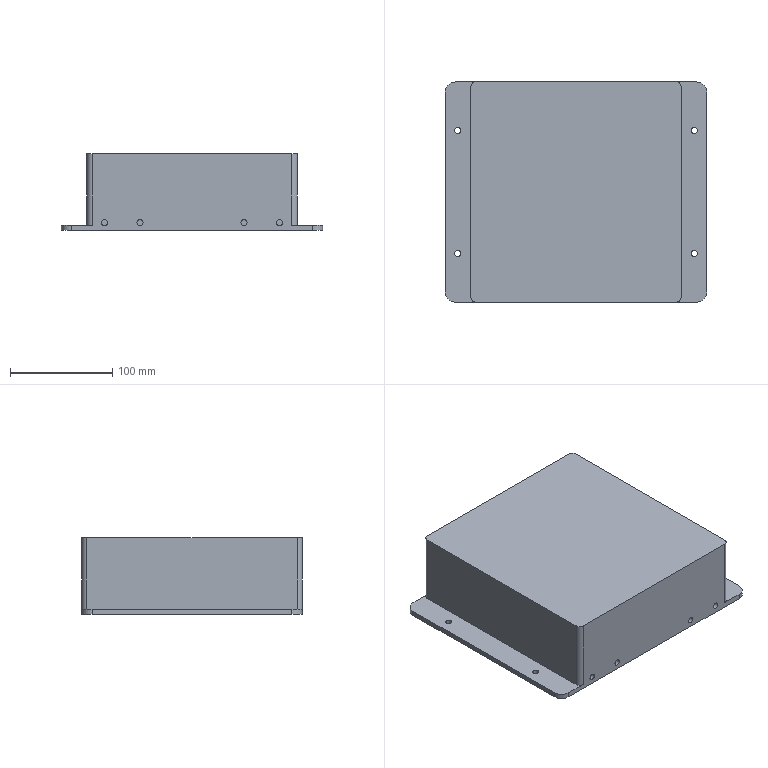Part | 1 solid | 46 faces | box 255 x 215 x 75 mm | volume 559118 mm3 | cylinder 29 | plane 17 | commonest cylinder face diameters 6 x16 10 x9 20 x4
STEP:
#1=CARTESIAN_POINT('',(102.5,102.5,0.));
#2=VERTEX_POINT('',#1);
#3=CARTESIAN_POINT('',(102.5,-102.5,0.));
#4=VERTEX_POINT('',#3);
#5=CARTESIAN_POINT('',(102.5,102.5,0.));
#6=DIRECTION('',(0.,-1.,0.));
#7=VECTOR('',#6,1000.);
#8=LINE('',#5,#7);
#9=EDGE_CURVE('',#2,#4,#8,.T.);
#10=ORIENTED_EDGE('',*,*,#9,.F.);
#11=CARTESIAN_POINT('',(97.5,107.5,0.));
#12=VERTEX_POINT('',#11);
#13=CARTESIAN_POINT('',(97.5,102.5,0.));
#14=DIRECTION('',(0.,0.,1.));
#15=DIRECTION('',(1.,0.,0.));
#16=AXIS2_PLACEMENT_3D('',#13,#14,#15);
#17=CIRCLE('',#16,5.);
#18=EDGE_CURVE('',#2,#12,#17,.T.);
#19=ORIENTED_EDGE('',*,*,#18,.T.);
#20=CARTESIAN_POINT('',(-97.5,107.5,0.));
#21=VERTEX_POINT('',#20);
#22=CARTESIAN_POINT('',(-97.5,107.5,0.));
#23=DIRECTION('',(1.,0.,0.));
#24=VECTOR('',#23,1000.);
#25=LINE('',#22,#24);
#26=EDGE_CURVE('',#21,#12,#25,.T.);
#27=ORIENTED_EDGE('',*,*,#26,.F.);
#28=CARTESIAN_POINT('',(-102.5,102.5,0.));
#29=VERTEX_POINT('',#28);
#30=CARTESIAN_POINT('',(-97.5,102.5,0.));
#31=DIRECTION('',(0.,0.,1.));
#32=DIRECTION('',(0.,1.,0.));
#33=AXIS2_PLACEMENT_3D('',#30,#31,#32);
#34=CIRCLE('',#33,5.);
#35=EDGE_CURVE('',#21,#29,#34,.T.);
#36=ORIENTED_EDGE('',*,*,#35,.T.);
#37=CARTESIAN_POINT('',(-102.5,-102.5,0.));
#38=VERTEX_POINT('',#37);
#39=CARTESIAN_POINT('',(-102.5,-102.5,0.));
#40=DIRECTION('',(0.,1.,0.));
#41=VECTOR('',#40,1000.);
#42=LINE('',#39,#41);
#43=EDGE_CURVE('',#38,#29,#42,.T.);
#44=ORIENTED_EDGE('',*,*,#43,.F.);
#45=CARTESIAN_POINT('',(-97.5,-107.5,0.));
#46=VERTEX_POINT('',#45);
#47=CARTESIAN_POINT('',(-97.5,-102.5,0.));
#48=DIRECTION('',(0.,0.,1.));
#49=DIRECTION('',(-1.,0.,0.));
#50=AXIS2_PLACEMENT_3D('',#47,#48,#49);
#51=CIRCLE('',#50,5.);
#52=EDGE_CURVE('',#38,#46,#51,.T.);
#53=ORIENTED_EDGE('',*,*,#52,.T.);
#54=CARTESIAN_POINT('',(97.5,-107.5,0.));
#55=VERTEX_POINT('',#54);
#56=CARTESIAN_POINT('',(97.5,-107.5,0.));
#57=DIRECTION('',(-1.,0.,0.));
#58=VECTOR('',#57,1000.);
#59=LINE('',#56,#58);
#60=EDGE_CURVE('',#55,#46,#59,.T.);
#61=ORIENTED_EDGE('',*,*,#60,.F.);
#62=CARTESIAN_POINT('',(97.5,-102.5,0.));
#63=DIRECTION('',(0.,0.,1.));
#64=DIRECTION('',(0.,-1.,0.));
#65=AXIS2_PLACEMENT_3D('',#62,#63,#64);
#66=CIRCLE('',#65,5.);
#67=EDGE_CURVE('',#55,#4,#66,.T.);
#68=ORIENTED_EDGE('',*,*,#67,.T.);
#69=EDGE_LOOP('',(#10,#19,#27,#36,#44,#53,#61,#68));
#70=FACE_BOUND('',#69,.T.);
#71=CARTESIAN_POINT('',(0.,5.,0.));
#72=DIRECTION('',(0.,0.,-1.));
#73=DIRECTION('',(1.,0.,0.));
#74=AXIS2_PLACEMENT_3D('',#71,#72,#73);
#75=PLANE('',#74);
#76=ADVANCED_FACE('',(#70),#75,.F.);
#77=CARTESIAN_POINT('',(97.5,-107.5,-70.));
#78=VERTEX_POINT('',#77);
#79=CARTESIAN_POINT('',(97.5,-107.5,-70.));
#80=DIRECTION('',(0.,0.,1.));
#81=VECTOR('',#80,1000.);
#82=LINE('',#79,#81);
#83=EDGE_CURVE('',#78,#55,#82,.T.);
#84=ORIENTED_EDGE('',*,*,#83,.F.);
#85=CARTESIAN_POINT('',(102.5,-102.5,-70.));
#86=VERTEX_POINT('',#85);
#87=CARTESIAN_POINT('',(97.5,-102.5,-70.));
#88=DIRECTION('',(0.,0.,-1.));
#89=DIRECTION('',(1.,0.,0.));
#90=AXIS2_PLACEMENT_3D('',#87,#88,#89);
#91=CIRCLE('',#90,5.);
#92=EDGE_CURVE('',#86,#78,#91,.T.);
#93=ORIENTED_EDGE('',*,*,#92,.F.);
#94=CARTESIAN_POINT('',(102.5,-102.5,-70.));
#95=DIRECTION('',(0.,0.,1.));
#96=VECTOR('',#95,1000.);
#97=LINE('',#94,#96);
#98=EDGE_CURVE('',#86,#4,#97,.T.);
#99=ORIENTED_EDGE('',*,*,#98,.T.);
#100=ORIENTED_EDGE('',*,*,#67,.F.);
#101=EDGE_LOOP('',(#84,#93,#99,#100));
#102=FACE_BOUND('',#101,.T.);
#103=CARTESIAN_POINT('',(97.5,-102.5,-172.77));
#104=DIRECTION('',(0.,0.,1.));
#105=DIRECTION('',(0.,1.,0.));
#106=AXIS2_PLACEMENT_3D('',#103,#104,#105);
#107=CYLINDRICAL_SURFACE('',#106,5.);
#108=ADVANCED_FACE('',(#102),#107,.T.);
#109=CARTESIAN_POINT('',(102.5,102.5,-70.));
#110=VERTEX_POINT('',#109);
#111=CARTESIAN_POINT('',(102.5,102.5,-70.));
#112=DIRECTION('',(0.,-1.,0.));
#113=VECTOR('',#112,1000.);
#114=LINE('',#111,#113);
#115=EDGE_CURVE('',#110,#86,#114,.T.);
#116=ORIENTED_EDGE('',*,*,#115,.F.);
#117=CARTESIAN_POINT('',(102.5,102.5,-70.));
#118=DIRECTION('',(0.,0.,1.));
#119=VECTOR('',#118,1000.);
#120=LINE('',#117,#119);
#121=EDGE_CURVE('',#110,#2,#120,.T.);
#122=ORIENTED_EDGE('',*,*,#121,.T.);
#123=ORIENTED_EDGE('',*,*,#9,.T.);
#124=ORIENTED_EDGE('',*,*,#98,.F.);
#125=EDGE_LOOP('',(#116,#122,#123,#124));
#126=FACE_BOUND('',#125,.T.);
#127=CARTESIAN_POINT('',(102.5,107.5,0.));
#128=DIRECTION('',(1.,0.,0.));
#129=DIRECTION('',(0.,1.,0.));
#130=AXIS2_PLACEMENT_3D('',#127,#128,#129);
#131=PLANE('',#130);
#132=ADVANCED_FACE('',(#126),#131,.T.);
#133=ORIENTED_EDGE('',*,*,#121,.F.);
#134=CARTESIAN_POINT('',(97.5,107.5,-70.));
#135=VERTEX_POINT('',#134);
#136=CARTESIAN_POINT('',(97.5,102.5,-70.));
#137=DIRECTION('',(0.,0.,-1.));
#138=DIRECTION('',(0.,1.,0.));
#139=AXIS2_PLACEMENT_3D('',#136,#137,#138);
#140=CIRCLE('',#139,5.);
#141=EDGE_CURVE('',#135,#110,#140,.T.);
#142=ORIENTED_EDGE('',*,*,#141,.F.);
#143=CARTESIAN_POINT('',(97.5,107.5,-70.));
#144=DIRECTION('',(0.,0.,1.));
#145=VECTOR('',#144,1000.);
#146=LINE('',#143,#145);
#147=EDGE_CURVE('',#135,#12,#146,.T.);
#148=ORIENTED_EDGE('',*,*,#147,.T.);
#149=ORIENTED_EDGE('',*,*,#18,.F.);
#150=EDGE_LOOP('',(#133,#142,#148,#149));
#151=FACE_BOUND('',#150,.T.);
#152=CARTESIAN_POINT('',(97.5,102.5,-172.77));
#153=DIRECTION('',(0.,0.,1.));
#154=DIRECTION('',(-1.,0.,0.));
#155=AXIS2_PLACEMENT_3D('',#152,#153,#154);
#156=CYLINDRICAL_SURFACE('',#155,5.);
#157=ADVANCED_FACE('',(#151),#156,.T.);
#158=ORIENTED_EDGE('',*,*,#26,.T.);
#159=ORIENTED_EDGE('',*,*,#147,.F.);
#160=CARTESIAN_POINT('',(117.5,107.5,-70.));
#161=VERTEX_POINT('',#160);
#162=CARTESIAN_POINT('',(97.5,107.5,-70.));
#163=DIRECTION('',(1.,0.,0.));
#164=VECTOR('',#163,1000.);
#165=LINE('',#162,#164);
#166=EDGE_CURVE('',#135,#161,#165,.T.);
#167=ORIENTED_EDGE('',*,*,#166,.T.);
#168=CARTESIAN_POINT('',(117.5,107.5,-75.));
#169=VERTEX_POINT('',#168);
#170=CARTESIAN_POINT('',(117.5,107.5,-75.));
#171=DIRECTION('',(0.,0.,1.));
#172=VECTOR('',#171,1000.);
#173=LINE('',#170,#172);
#174=EDGE_CURVE('',#169,#161,#173,.T.);
#175=ORIENTED_EDGE('',*,*,#174,.F.);
#176=CARTESIAN_POINT('',(70.,107.5,-75.));
#177=VERTEX_POINT('',#176);
#178=CARTESIAN_POINT('',(70.,107.5,-75.));
#179=DIRECTION('',(1.,0.,0.));
#180=VECTOR('',#179,1000.);
#181=LINE('',#178,#180);
#182=EDGE_CURVE('',#177,#169,#181,.T.);
#183=ORIENTED_EDGE('',*,*,#182,.F.);
#184=CARTESIAN_POINT('',(70.,107.5,-70.));
#185=VERTEX_POINT('',#184);
#186=CARTESIAN_POINT('',(70.,107.5,-75.));
#187=DIRECTION('',(0.,0.,1.));
#188=VECTOR('',#187,1000.);
#189=LINE('',#186,#188);
#190=EDGE_CURVE('',#177,#185,#189,.T.);
#191=ORIENTED_EDGE('',*,*,#190,.T.);
#192=CARTESIAN_POINT('',(60.,107.5,-70.));
#193=VERTEX_POINT('',#192);
#194=CARTESIAN_POINT('',(65.,107.5,-70.));
#195=DIRECTION('',(0.,1.,0.));
#196=DIRECTION('',(-1.,0.,0.));
#197=AXIS2_PLACEMENT_3D('',#194,#195,#196);
#198=CIRCLE('',#197,5.);
#199=EDGE_CURVE('',#193,#185,#198,.T.);
#200=ORIENTED_EDGE('',*,*,#199,.F.);
#201=CARTESIAN_POINT('',(60.,107.5,-75.));
#202=VERTEX_POINT('',#201);
#203=CARTESIAN_POINT('',(60.,107.5,-75.));
#204=DIRECTION('',(0.,0.,1.));
#205=VECTOR('',#204,1000.);
#206=LINE('',#203,#205);
#207=EDGE_CURVE('',#202,#193,#206,.T.);
#208=ORIENTED_EDGE('',*,*,#207,.F.);
#209=CARTESIAN_POINT('',(-117.5,107.5,-75.));
#210=VERTEX_POINT('',#209);
#211=CARTESIAN_POINT('',(-117.5,107.5,-75.));
#212=DIRECTION('',(1.,0.,0.));
#213=VECTOR('',#212,1000.);
#214=LINE('',#211,#213);
#215=EDGE_CURVE('',#210,#202,#214,.T.);
#216=ORIENTED_EDGE('',*,*,#215,.F.);
#217=CARTESIAN_POINT('',(-117.5,107.5,-70.));
#218=VERTEX_POINT('',#217);
#219=CARTESIAN_POINT('',(-117.5,107.5,-75.));
#220=DIRECTION('',(0.,0.,1.));
#221=VECTOR('',#220,1000.);
#222=LINE('',#219,#221);
#223=EDGE_CURVE('',#210,#218,#222,.T.);
#224=ORIENTED_EDGE('',*,*,#223,.T.);
#225=CARTESIAN_POINT('',(-97.5,107.5,-70.));
#226=VERTEX_POINT('',#225);
#227=CARTESIAN_POINT('',(-117.5,107.5,-70.));
#228=DIRECTION('',(1.,0.,0.));
#229=VECTOR('',#228,1000.);
#230=LINE('',#227,#229);
#231=EDGE_CURVE('',#218,#226,#230,.T.);
#232=ORIENTED_EDGE('',*,*,#231,.T.);
#233=CARTESIAN_POINT('',(-97.5,107.5,-70.));
#234=DIRECTION('',(0.,0.,1.));
#235=VECTOR('',#234,1000.);
#236=LINE('',#233,#235);
#237=EDGE_CURVE('',#226,#21,#236,.T.);
#238=ORIENTED_EDGE('',*,*,#237,.T.);
#239=EDGE_LOOP('',(#158,#159,#167,#175,#183,#191,#200,#208,#216,#224,#232,#238));
#240=FACE_BOUND('',#239,.T.);
#241=CARTESIAN_POINT('',(-102.5,107.5,0.));
#242=DIRECTION('',(0.,1.,0.));
#243=DIRECTION('',(-1.,0.,0.));
#244=AXIS2_PLACEMENT_3D('',#241,#242,#243);
#245=PLANE('',#244);
#246=ADVANCED_FACE('',(#240),#245,.T.);
#247=ORIENTED_EDGE('',*,*,#237,.F.);
#248=CARTESIAN_POINT('',(-102.5,102.5,-70.));
#249=VERTEX_POINT('',#248);
#250=CARTESIAN_POINT('',(-97.5,102.5,-70.));
#251=DIRECTION('',(0.,0.,-1.));
#252=DIRECTION('',(-1.,0.,0.));
#253=AXIS2_PLACEMENT_3D('',#250,#251,#252);
#254=CIRCLE('',#253,5.);
#255=EDGE_CURVE('',#249,#226,#254,.T.);
#256=ORIENTED_EDGE('',*,*,#255,.F.);
#257=CARTESIAN_POINT('',(-102.5,102.5,-70.));
#258=DIRECTION('',(0.,0.,1.));
#259=VECTOR('',#258,1000.);
#260=LINE('',#257,#259);
#261=EDGE_CURVE('',#249,#29,#260,.T.);
#262=ORIENTED_EDGE('',*,*,#261,.T.);
#263=ORIENTED_EDGE('',*,*,#35,.F.);
#264=EDGE_LOOP('',(#247,#256,#262,#263));
#265=FACE_BOUND('',#264,.T.);
#266=CARTESIAN_POINT('',(-97.5,102.5,-172.77));
#267=DIRECTION('',(0.,0.,1.));
#268=DIRECTION('',(0.,-1.,0.));
#269=AXIS2_PLACEMENT_3D('',#266,#267,#268);
#270=CYLINDRICAL_SURFACE('',#269,5.);
#271=ADVANCED_FACE('',(#265),#270,.T.);
#272=ORIENTED_EDGE('',*,*,#43,.T.);
#273=ORIENTED_EDGE('',*,*,#261,.F.);
#274=CARTESIAN_POINT('',(-102.5,-102.5,-70.));
#275=VERTEX_POINT('',#274);
#276=CARTESIAN_POINT('',(-102.5,-102.5,-70.));
#277=DIRECTION('',(0.,1.,0.));
#278=VECTOR('',#277,1000.);
#279=LINE('',#276,#278);
#280=EDGE_CURVE('',#275,#249,#279,.T.);
#281=ORIENTED_EDGE('',*,*,#280,.F.);
#282=CARTESIAN_POINT('',(-102.5,-102.5,-70.));
#283=DIRECTION('',(0.,0.,1.));
#284=VECTOR('',#283,1000.);
#285=LINE('',#282,#284);
#286=EDGE_CURVE('',#275,#38,#285,.T.);
#287=ORIENTED_EDGE('',*,*,#286,.T.);
#288=EDGE_LOOP('',(#272,#273,#281,#287));
#289=FACE_BOUND('',#288,.T.);
#290=CARTESIAN_POINT('',(-102.5,-97.5,0.));
#291=DIRECTION('',(-1.,0.,0.));
#292=DIRECTION('',(0.,-1.,0.));
#293=AXIS2_PLACEMENT_3D('',#290,#291,#292);
#294=PLANE('',#293);
#295=ADVANCED_FACE('',(#289),#294,.T.);
#296=ORIENTED_EDGE('',*,*,#286,.F.);
#297=CARTESIAN_POINT('',(-97.5,-107.5,-70.));
#298=VERTEX_POINT('',#297);
#299=CARTESIAN_POINT('',(-97.5,-102.5,-70.));
#300=DIRECTION('',(0.,0.,-1.));
#301=DIRECTION('',(0.,-1.,0.));
#302=AXIS2_PLACEMENT_3D('',#299,#300,#301);
#303=CIRCLE('',#302,5.);
#304=EDGE_CURVE('',#298,#275,#303,.T.);
#305=ORIENTED_EDGE('',*,*,#304,.F.);
#306=CARTESIAN_POINT('',(-97.5,-107.5,-70.));
#307=DIRECTION('',(0.,0.,1.));
#308=VECTOR('',#307,1000.);
#309=LINE('',#306,#308);
#310=EDGE_CURVE('',#298,#46,#309,.T.);
#311=ORIENTED_EDGE('',*,*,#310,.T.);
#312=ORIENTED_EDGE('',*,*,#52,.F.);
#313=EDGE_LOOP('',(#296,#305,#311,#312));
#314=FACE_BOUND('',#313,.T.);
#315=CARTESIAN_POINT('',(-97.5,-102.5,-172.77));
#316=DIRECTION('',(0.,0.,1.));
#317=DIRECTION('',(1.,0.,0.));
#318=AXIS2_PLACEMENT_3D('',#315,#316,#317);
#319=CYLINDRICAL_SURFACE('',#318,5.);
#320=ADVANCED_FACE('',(#314),#319,.T.);
#321=ORIENTED_EDGE('',*,*,#60,.T.);
#322=ORIENTED_EDGE('',*,*,#310,.F.);
#323=CARTESIAN_POINT('',(-117.5,-107.5,-70.));
#324=VERTEX_POINT('',#323);
#325=CARTESIAN_POINT('',(-97.5,-107.5,-70.));
#326=DIRECTION('',(-1.,0.,0.));
#327=VECTOR('',#326,1000.);
#328=LINE('',#325,#327);
#329=EDGE_CURVE('',#298,#324,#328,.T.);
#330=ORIENTED_EDGE('',*,*,#329,.T.);
#331=CARTESIAN_POINT('',(-117.5,-107.5,-75.));
#332=VERTEX_POINT('',#331);
#333=CARTESIAN_POINT('',(-117.5,-107.5,-75.));
#334=DIRECTION('',(0.,0.,1.));
#335=VECTOR('',#334,1000.);
#336=LINE('',#333,#335);
#337=EDGE_CURVE('',#332,#324,#336,.T.);
#338=ORIENTED_EDGE('',*,*,#337,.F.);
#339=CARTESIAN_POINT('',(117.5,-107.5,-75.));
#340=VERTEX_POINT('',#339);
#341=CARTESIAN_POINT('',(117.5,-107.5,-75.));
#342=DIRECTION('',(-1.,0.,0.));
#343=VECTOR('',#342,1000.);
#344=LINE('',#341,#343);
#345=EDGE_CURVE('',#340,#332,#344,.T.);
#346=ORIENTED_EDGE('',*,*,#345,.F.);
#347=CARTESIAN_POINT('',(117.5,-107.5,-70.));
#348=VERTEX_POINT('',#347);
#349=CARTESIAN_POINT('',(117.5,-107.5,-75.));
#350=DIRECTION('',(0.,0.,1.));
#351=VECTOR('',#350,1000.);
#352=LINE('',#349,#351);
#353=EDGE_CURVE('',#340,#348,#352,.T.);
#354=ORIENTED_EDGE('',*,*,#353,.T.);
#355=CARTESIAN_POINT('',(117.5,-107.5,-70.));
#356=DIRECTION('',(-1.,0.,0.));
#357=VECTOR('',#356,1000.);
#358=LINE('',#355,#357);
#359=EDGE_CURVE('',#348,#78,#358,.T.);
#360=ORIENTED_EDGE('',*,*,#359,.T.);
#361=ORIENTED_EDGE('',*,*,#83,.T.);
#362=EDGE_LOOP('',(#321,#322,#330,#338,#346,#354,#360,#361));
#363=FACE_BOUND('',#362,.T.);
#364=CARTESIAN_POINT('',(-82.25,-107.5,-67.35));
#365=VERTEX_POINT('',#364);
#366=CARTESIAN_POINT('',(-88.25,-107.5,-67.35));
#367=VERTEX_POINT('',#366);
#368=CARTESIAN_POINT('',(-85.25,-107.5,-67.35));
#369=DIRECTION('',(0.,-1.,0.));
#370=DIRECTION('',(1.,0.,0.));
#371=AXIS2_PLACEMENT_3D('',#368,#369,#370);
#372=CIRCLE('',#371,3.);
#373=EDGE_CURVE('',#365,#367,#372,.T.);
#374=ORIENTED_EDGE('',*,*,#373,.F.);
#375=CARTESIAN_POINT('',(-85.25,-107.5,-67.35));
#376=DIRECTION('',(0.,-1.,0.));
#377=DIRECTION('',(-1.,0.,0.));
#378=AXIS2_PLACEMENT_3D('',#375,#376,#377);
#379=CIRCLE('',#378,3.);
#380=EDGE_CURVE('',#367,#365,#379,.T.);
#381=ORIENTED_EDGE('',*,*,#380,.F.);
#382=EDGE_LOOP('',(#374,#381));
#383=FACE_BOUND('',#382,.T.);
#384=CARTESIAN_POINT('',(53.75,-107.5,-67.35));
#385=VERTEX_POINT('',#384);
#386=CARTESIAN_POINT('',(47.75,-107.5,-67.35));
#387=VERTEX_POINT('',#386);
#388=CARTESIAN_POINT('',(50.75,-107.5,-67.35));
#389=DIRECTION('',(0.,-1.,0.));
#390=DIRECTION('',(1.,0.,0.));
#391=AXIS2_PLACEMENT_3D('',#388,#389,#390);
#392=CIRCLE('',#391,3.);
#393=EDGE_CURVE('',#385,#387,#392,.T.);
#394=ORIENTED_EDGE('',*,*,#393,.F.);
#395=CARTESIAN_POINT('',(50.75,-107.5,-67.35));
#396=DIRECTION('',(0.,-1.,0.));
#397=DIRECTION('',(-1.,0.,0.));
#398=AXIS2_PLACEMENT_3D('',#395,#396,#397);
#399=CIRCLE('',#398,3.);
#400=EDGE_CURVE('',#387,#385,#399,.T.);
#401=ORIENTED_EDGE('',*,*,#400,.F.);
#402=EDGE_LOOP('',(#394,#401));
#403=FACE_BOUND('',#402,.T.);
#404=CARTESIAN_POINT('',(88.25,-107.5,-67.35));
#405=VERTEX_POINT('',#404);
#406=CARTESIAN_POINT('',(82.25,-107.5,-67.35));
#407=VERTEX_POINT('',#406);
#408=CARTESIAN_POINT('',(85.25,-107.5,-67.35));
#409=DIRECTION('',(0.,-1.,0.));
#410=DIRECTION('',(1.,0.,0.));
#411=AXIS2_PLACEMENT_3D('',#408,#409,#410);
#412=CIRCLE('',#411,3.);
#413=EDGE_CURVE('',#405,#407,#412,.T.);
#414=ORIENTED_EDGE('',*,*,#413,.F.);
#415=CARTESIAN_POINT('',(85.25,-107.5,-67.35));
#416=DIRECTION('',(0.,-1.,0.));
#417=DIRECTION('',(-1.,0.,0.));
#418=AXIS2_PLACEMENT_3D('',#415,#416,#417);
#419=CIRCLE('',#418,3.);
#420=EDGE_CURVE('',#407,#405,#419,.T.);
#421=ORIENTED_EDGE('',*,*,#420,.F.);
#422=EDGE_LOOP('',(#414,#421));
#423=FACE_BOUND('',#422,.T.);
#424=CARTESIAN_POINT('',(-47.75,-107.5,-67.35));
#425=VERTEX_POINT('',#424);
#426=CARTESIAN_POINT('',(-53.75,-107.5,-67.35));
#427=VERTEX_POINT('',#426);
#428=CARTESIAN_POINT('',(-50.75,-107.5,-67.35));
#429=DIRECTION('',(0.,-1.,0.));
#430=DIRECTION('',(1.,0.,0.));
#431=AXIS2_PLACEMENT_3D('',#428,#429,#430);
#432=CIRCLE('',#431,3.);
#433=EDGE_CURVE('',#425,#427,#432,.T.);
#434=ORIENTED_EDGE('',*,*,#433,.F.);
#435=CARTESIAN_POINT('',(-50.75,-107.5,-67.35));
#436=DIRECTION('',(0.,-1.,0.));
#437=DIRECTION('',(-1.,0.,0.));
#438=AXIS2_PLACEMENT_3D('',#435,#436,#437);
#439=CIRCLE('',#438,3.);
#440=EDGE_CURVE('',#427,#425,#439,.T.);
#441=ORIENTED_EDGE('',*,*,#440,.F.);
#442=EDGE_LOOP('',(#434,#441));
#443=FACE_BOUND('',#442,.T.);
#444=CARTESIAN_POINT('',(102.5,-107.5,0.));
#445=DIRECTION('',(0.,-1.,0.));
#446=DIRECTION('',(1.,0.,0.));
#447=AXIS2_PLACEMENT_3D('',#444,#445,#446);
#448=PLANE('',#447);
#449=ADVANCED_FACE('',(#363,#383,#403,#423,#443),#448,.T.);
#450=CARTESIAN_POINT('',(-47.75,-102.5,-67.35));
#451=VERTEX_POINT('',#450);
#452=CARTESIAN_POINT('',(-47.75,-107.5,-67.35));
#453=DIRECTION('',(0.,1.,0.));
#454=VECTOR('',#453,1000.);
#455=LINE('',#452,#454);
#456=EDGE_CURVE('',#451,#425,#455,.F.);
#457=ORIENTED_EDGE('',*,*,#456,.F.);
#458=CARTESIAN_POINT('',(-53.75,-102.5,-67.35));
#459=VERTEX_POINT('',#458);
#460=CARTESIAN_POINT('',(-50.75,-102.5,-67.35));
#461=DIRECTION('',(0.,-1.,0.));
#462=DIRECTION('',(-1.,0.,0.));
#463=AXIS2_PLACEMENT_3D('',#460,#461,#462);
#464=CIRCLE('',#463,3.);
#465=EDGE_CURVE('',#459,#451,#464,.T.);
#466=ORIENTED_EDGE('',*,*,#465,.F.);
#467=CARTESIAN_POINT('',(-53.75,-107.5,-67.35));
#468=DIRECTION('',(0.,1.,0.));
#469=VECTOR('',#468,1000.);
#470=LINE('',#467,#469);
#471=EDGE_CURVE('',#459,#427,#470,.F.);
#472=ORIENTED_EDGE('',*,*,#471,.T.);
#473=ORIENTED_EDGE('',*,*,#440,.T.);
#474=EDGE_LOOP('',(#457,#466,#472,#473));
#475=FACE_BOUND('',#474,.T.);
#476=CARTESIAN_POINT('',(-50.75,-107.5,-67.35));
#477=DIRECTION('',(0.,-1.,0.));
#478=DIRECTION('',(1.,0.,0.));
#479=AXIS2_PLACEMENT_3D('',#476,#477,#478);
#480=CYLINDRICAL_SURFACE('',#479,3.);
#481=ADVANCED_FACE('',(#475),#480,.F.);
#482=ORIENTED_EDGE('',*,*,#471,.F.);
#483=CARTESIAN_POINT('',(-50.75,-102.5,-67.35));
#484=DIRECTION('',(0.,-1.,0.));
#485=DIRECTION('',(1.,0.,0.));
#486=AXIS2_PLACEMENT_3D('',#483,#484,#485);
#487=CIRCLE('',#486,3.);
#488=EDGE_CURVE('',#451,#459,#487,.T.);
#489=ORIENTED_EDGE('',*,*,#488,.F.);
#490=ORIENTED_EDGE('',*,*,#456,.T.);
#491=ORIENTED_EDGE('',*,*,#433,.T.);
#492=EDGE_LOOP('',(#482,#489,#490,#491));
#493=FACE_BOUND('',#492,.T.);
#494=CARTESIAN_POINT('',(-50.75,-107.5,-67.35));
#495=DIRECTION('',(0.,-1.,0.));
#496=DIRECTION('',(1.,0.,0.));
#497=AXIS2_PLACEMENT_3D('',#494,#495,#496);
#498=CYLINDRICAL_SURFACE('',#497,3.);
#499=ADVANCED_FACE('',(#493),#498,.F.);
#500=CARTESIAN_POINT('',(92.5,-102.5,-5.));
#501=VERTEX_POINT('',#500);
#502=CARTESIAN_POINT('',(-92.5,-102.5,-5.));
#503=VERTEX_POINT('',#502);
#504=CARTESIAN_POINT('',(92.5,-102.5,-5.));
#505=DIRECTION('',(-1.,0.,0.));
#506=VECTOR('',#505,1000.);
#507=LINE('',#504,#506);
#508=EDGE_CURVE('',#501,#503,#507,.T.);
#509=ORIENTED_EDGE('',*,*,#508,.F.);
#510=CARTESIAN_POINT('',(92.5,-102.5,-75.));
#511=VERTEX_POINT('',#510);
#512=CARTESIAN_POINT('',(92.5,-102.5,-75.));
#513=DIRECTION('',(0.,0.,1.));
#514=VECTOR('',#513,1000.);
#515=LINE('',#512,#514);
#516=EDGE_CURVE('',#511,#501,#515,.T.);
#517=ORIENTED_EDGE('',*,*,#516,.F.);
#518=CARTESIAN_POINT('',(-92.5,-102.5,-75.));
#519=VERTEX_POINT('',#518);
#520=CARTESIAN_POINT('',(92.5,-102.5,-75.));
#521=DIRECTION('',(-1.,0.,0.));
#522=VECTOR('',#521,1000.);
#523=LINE('',#520,#522);
#524=EDGE_CURVE('',#511,#519,#523,.T.);
#525=ORIENTED_EDGE('',*,*,#524,.T.);
#526=CARTESIAN_POINT('',(-92.5,-102.5,-75.));
#527=DIRECTION('',(0.,0.,1.));
#528=VECTOR('',#527,1000.);
#529=LINE('',#526,#528);
#530=EDGE_CURVE('',#519,#503,#529,.T.);
#531=ORIENTED_EDGE('',*,*,#530,.T.);
#532=EDGE_LOOP('',(#509,#517,#525,#531));
#533=FACE_BOUND('',#532,.T.);
#534=CARTESIAN_POINT('',(-82.25,-102.5,-67.35));
#535=VERTEX_POINT('',#534);
#536=CARTESIAN_POINT('',(-88.25,-102.5,-67.35));
#537=VERTEX_POINT('',#536);
#538=CARTESIAN_POINT('',(-85.25,-102.5,-67.35));
#539=DIRECTION('',(0.,-1.,0.));
#540=DIRECTION('',(1.,0.,0.));
#541=AXIS2_PLACEMENT_3D('',#538,#539,#540);
#542=CIRCLE('',#541,3.);
#543=EDGE_CURVE('',#535,#537,#542,.T.);
#544=ORIENTED_EDGE('',*,*,#543,.T.);
#545=CARTESIAN_POINT('',(-85.25,-102.5,-67.35));
#546=DIRECTION('',(0.,-1.,0.));
#547=DIRECTION('',(-1.,0.,0.));
#548=AXIS2_PLACEMENT_3D('',#545,#546,#547);
#549=CIRCLE('',#548,3.);
#550=EDGE_CURVE('',#537,#535,#549,.T.);
#551=ORIENTED_EDGE('',*,*,#550,.T.);
#552=EDGE_LOOP('',(#544,#551));
#553=FACE_BOUND('',#552,.T.);
#554=CARTESIAN_POINT('',(53.75,-102.5,-67.35));
#555=VERTEX_POINT('',#554);
#556=CARTESIAN_POINT('',(47.75,-102.5,-67.35));
#557=VERTEX_POINT('',#556);
#558=CARTESIAN_POINT('',(50.75,-102.5,-67.35));
#559=DIRECTION('',(0.,-1.,0.));
#560=DIRECTION('',(1.,0.,0.));
#561=AXIS2_PLACEMENT_3D('',#558,#559,#560);
#562=CIRCLE('',#561,3.);
#563=EDGE_CURVE('',#555,#557,#562,.T.);
#564=ORIENTED_EDGE('',*,*,#563,.T.);
#565=CARTESIAN_POINT('',(50.75,-102.5,-67.35));
#566=DIRECTION('',(0.,-1.,0.));
#567=DIRECTION('',(-1.,0.,0.));
#568=AXIS2_PLACEMENT_3D('',#565,#566,#567);
#569=CIRCLE('',#568,3.);
#570=EDGE_CURVE('',#557,#555,#569,.T.);
#571=ORIENTED_EDGE('',*,*,#570,.T.);
#572=EDGE_LOOP('',(#564,#571));
#573=FACE_BOUND('',#572,.T.);
#574=CARTESIAN_POINT('',(88.25,-102.5,-67.35));
#575=VERTEX_POINT('',#574);
#576=CARTESIAN_POINT('',(82.25,-102.5,-67.35));
#577=VERTEX_POINT('',#576);
#578=CARTESIAN_POINT('',(85.25,-102.5,-67.35));
#579=DIRECTION('',(0.,-1.,0.));
#580=DIRECTION('',(1.,0.,0.));
#581=AXIS2_PLACEMENT_3D('',#578,#579,#580);
#582=CIRCLE('',#581,3.);
#583=EDGE_CURVE('',#575,#577,#582,.T.);
#584=ORIENTED_EDGE('',*,*,#583,.T.);
#585=CARTESIAN_POINT('',(85.25,-102.5,-67.35));
#586=DIRECTION('',(0.,-1.,0.));
#587=DIRECTION('',(-1.,0.,0.));
#588=AXIS2_PLACEMENT_3D('',#585,#586,#587);
#589=CIRCLE('',#588,3.);
#590=EDGE_CURVE('',#577,#575,#589,.T.);
#591=ORIENTED_EDGE('',*,*,#590,.T.);
#592=EDGE_LOOP('',(#584,#591));
#593=FACE_BOUND('',#592,.T.);
#594=ORIENTED_EDGE('',*,*,#488,.T.);
#595=ORIENTED_EDGE('',*,*,#465,.T.);
#596=EDGE_LOOP('',(#594,#595));
#597=FACE_BOUND('',#596,.T.);
#598=CARTESIAN_POINT('',(102.5,-102.5,0.));
#599=DIRECTION('',(0.,-1.,0.));
#600=DIRECTION('',(1.,0.,0.));
#601=AXIS2_PLACEMENT_3D('',#598,#599,#600);
#602=PLANE('',#601);
#603=ADVANCED_FACE('',(#533,#553,#573,#593,#597),#602,.F.);
#604=CARTESIAN_POINT('',(-82.25,-107.5,-67.35));
#605=DIRECTION('',(0.,1.,0.));
#606=VECTOR('',#605,1000.);
#607=LINE('',#604,#606);
#608=EDGE_CURVE('',#535,#365,#607,.F.);
#609=ORIENTED_EDGE('',*,*,#608,.F.);
#610=ORIENTED_EDGE('',*,*,#550,.F.);
#611=CARTESIAN_POINT('',(-88.25,-107.5,-67.35));
#612=DIRECTION('',(0.,1.,0.));
#613=VECTOR('',#612,1000.);
#614=LINE('',#611,#613);
#615=EDGE_CURVE('',#537,#367,#614,.F.);
#616=ORIENTED_EDGE('',*,*,#615,.T.);
#617=ORIENTED_EDGE('',*,*,#380,.T.);
#618=EDGE_LOOP('',(#609,#610,#616,#617));
#619=FACE_BOUND('',#618,.T.);
#620=CARTESIAN_POINT('',(-85.25,-107.5,-67.35));
#621=DIRECTION('',(0.,-1.,0.));
#622=DIRECTION('',(1.,0.,0.));
#623=AXIS2_PLACEMENT_3D('',#620,#621,#622);
#624=CYLINDRICAL_SURFACE('',#623,3.);
#625=ADVANCED_FACE('',(#619),#624,.F.);
#626=ORIENTED_EDGE('',*,*,#615,.F.);
#627=ORIENTED_EDGE('',*,*,#543,.F.);
#628=ORIENTED_EDGE('',*,*,#608,.T.);
#629=ORIENTED_EDGE('',*,*,#373,.T.);
#630=EDGE_LOOP('',(#626,#627,#628,#629));
#631=FACE_BOUND('',#630,.T.);
#632=CARTESIAN_POINT('',(-85.25,-107.5,-67.35));
#633=DIRECTION('',(0.,-1.,0.));
#634=DIRECTION('',(1.,0.,0.));
#635=AXIS2_PLACEMENT_3D('',#632,#633,#634);
#636=CYLINDRICAL_SURFACE('',#635,3.);
#637=ADVANCED_FACE('',(#631),#636,.F.);
#638=CARTESIAN_POINT('',(53.75,-107.5,-67.35));
#639=DIRECTION('',(0.,1.,0.));
#640=VECTOR('',#639,1000.);
#641=LINE('',#638,#640);
#642=EDGE_CURVE('',#555,#385,#641,.F.);
#643=ORIENTED_EDGE('',*,*,#642,.F.);
#644=ORIENTED_EDGE('',*,*,#570,.F.);
#645=CARTESIAN_POINT('',(47.75,-107.5,-67.35));
#646=DIRECTION('',(0.,1.,0.));
#647=VECTOR('',#646,1000.);
#648=LINE('',#645,#647);
#649=EDGE_CURVE('',#557,#387,#648,.F.);
#650=ORIENTED_EDGE('',*,*,#649,.T.);
#651=ORIENTED_EDGE('',*,*,#400,.T.);
#652=EDGE_LOOP('',(#643,#644,#650,#651));
#653=FACE_BOUND('',#652,.T.);
#654=CARTESIAN_POINT('',(50.75,-107.5,-67.35));
#655=DIRECTION('',(0.,-1.,0.));
#656=DIRECTION('',(1.,0.,0.));
#657=AXIS2_PLACEMENT_3D('',#654,#655,#656);
#658=CYLINDRICAL_SURFACE('',#657,3.);
#659=ADVANCED_FACE('',(#653),#658,.F.);
#660=ORIENTED_EDGE('',*,*,#649,.F.);
#661=ORIENTED_EDGE('',*,*,#563,.F.);
#662=ORIENTED_EDGE('',*,*,#642,.T.);
#663=ORIENTED_EDGE('',*,*,#393,.T.);
#664=EDGE_LOOP('',(#660,#661,#662,#663));
#665=FACE_BOUND('',#664,.T.);
#666=CARTESIAN_POINT('',(50.75,-107.5,-67.35));
#667=DIRECTION('',(0.,-1.,0.));
#668=DIRECTION('',(1.,0.,0.));
#669=AXIS2_PLACEMENT_3D('',#666,#667,#668);
#670=CYLINDRICAL_SURFACE('',#669,3.);
#671=ADVANCED_FACE('',(#665),#670,.F.);
#672=CARTESIAN_POINT('',(88.25,-107.5,-67.35));
#673=DIRECTION('',(0.,1.,0.));
#674=VECTOR('',#673,1000.);
#675=LINE('',#672,#674);
#676=EDGE_CURVE('',#575,#405,#675,.F.);
#677=ORIENTED_EDGE('',*,*,#676,.F.);
#678=ORIENTED_EDGE('',*,*,#590,.F.);
#679=CARTESIAN_POINT('',(82.25,-107.5,-67.35));
#680=DIRECTION('',(0.,1.,0.));
#681=VECTOR('',#680,1000.);
#682=LINE('',#679,#681);
#683=EDGE_CURVE('',#577,#407,#682,.F.);
#684=ORIENTED_EDGE('',*,*,#683,.T.);
#685=ORIENTED_EDGE('',*,*,#420,.T.);
#686=EDGE_LOOP('',(#677,#678,#684,#685));
#687=FACE_BOUND('',#686,.T.);
#688=CARTESIAN_POINT('',(85.25,-107.5,-67.35));
#689=DIRECTION('',(0.,-1.,0.));
#690=DIRECTION('',(1.,0.,0.));
#691=AXIS2_PLACEMENT_3D('',#688,#689,#690);
#692=CYLINDRICAL_SURFACE('',#691,3.);
#693=ADVANCED_FACE('',(#687),#692,.F.);
#694=ORIENTED_EDGE('',*,*,#683,.F.);
#695=ORIENTED_EDGE('',*,*,#583,.F.);
#696=ORIENTED_EDGE('',*,*,#676,.T.);
#697=ORIENTED_EDGE('',*,*,#413,.T.);
#698=EDGE_LOOP('',(#694,#695,#696,#697));
#699=FACE_BOUND('',#698,.T.);
#700=CARTESIAN_POINT('',(85.25,-107.5,-67.35));
#701=DIRECTION('',(0.,-1.,0.));
#702=DIRECTION('',(1.,0.,0.));
#703=AXIS2_PLACEMENT_3D('',#700,#701,#702);
#704=CYLINDRICAL_SURFACE('',#703,3.);
#705=ADVANCED_FACE('',(#699),#704,.F.);
#706=ORIENTED_EDGE('',*,*,#530,.F.);
#707=CARTESIAN_POINT('',(-97.5,-97.5,-75.));
#708=VERTEX_POINT('',#707);
#709=CARTESIAN_POINT('',(-92.5,-97.5,-75.));
#710=DIRECTION('',(0.,0.,1.));
#711=DIRECTION('',(-1.,0.,0.));
#712=AXIS2_PLACEMENT_3D('',#709,#710,#711);
#713=CIRCLE('',#712,5.);
#714=EDGE_CURVE('',#708,#519,#713,.T.);
#715=ORIENTED_EDGE('',*,*,#714,.F.);
#716=CARTESIAN_POINT('',(-97.5,-97.5,-5.));
#717=VERTEX_POINT('',#716);
#718=CARTESIAN_POINT('',(-97.5,-97.5,-75.));
#719=DIRECTION('',(0.,0.,1.));
#720=VECTOR('',#719,1000.);
#721=LINE('',#718,#720);
#722=EDGE_CURVE('',#708,#717,#721,.T.);
#723=ORIENTED_EDGE('',*,*,#722,.T.);
#724=CARTESIAN_POINT('',(-92.5,-97.5,-5.));
#725=DIRECTION('',(0.,0.,-1.));
#726=DIRECTION('',(0.,-1.,0.));
#727=AXIS2_PLACEMENT_3D('',#724,#725,#726);
#728=CIRCLE('',#727,5.);
#729=EDGE_CURVE('',#503,#717,#728,.T.);
#730=ORIENTED_EDGE('',*,*,#729,.F.);
#731=EDGE_LOOP('',(#706,#715,#723,#730));
#732=FACE_BOUND('',#731,.T.);
#733=CARTESIAN_POINT('',(-92.5,-97.5,-172.77));
#734=DIRECTION('',(0.,0.,1.));
#735=DIRECTION('',(1.,0.,0.));
#736=AXIS2_PLACEMENT_3D('',#733,#734,#735);
#737=CYLINDRICAL_SURFACE('',#736,5.);
#738=ADVANCED_FACE('',(#732),#737,.F.);
#739=CARTESIAN_POINT('',(-97.5,97.5,-5.));
#740=VERTEX_POINT('',#739);
#741=CARTESIAN_POINT('',(-97.5,-97.5,-5.));
#742=DIRECTION('',(0.,1.,0.));
#743=VECTOR('',#742,1000.);
#744=LINE('',#741,#743);
#745=EDGE_CURVE('',#717,#740,#744,.T.);
#746=ORIENTED_EDGE('',*,*,#745,.T.);
#747=CARTESIAN_POINT('',(-92.5,102.5,-5.));
#748=VERTEX_POINT('',#747);
#749=CARTESIAN_POINT('',(-92.5,97.5,-5.));
#750=DIRECTION('',(0.,0.,-1.));
#751=DIRECTION('',(-1.,0.,0.));
#752=AXIS2_PLACEMENT_3D('',#749,#750,#751);
#753=CIRCLE('',#752,5.);
#754=EDGE_CURVE('',#740,#748,#753,.T.);
#755=ORIENTED_EDGE('',*,*,#754,.T.);
#756=CARTESIAN_POINT('',(92.5,102.5,-5.));
#757=VERTEX_POINT('',#756);
#758=CARTESIAN_POINT('',(-92.5,102.5,-5.));
#759=DIRECTION('',(1.,0.,0.));
#760=VECTOR('',#759,1000.);
#761=LINE('',#758,#760);
#762=EDGE_CURVE('',#748,#757,#761,.T.);
#763=ORIENTED_EDGE('',*,*,#762,.T.);
#764=CARTESIAN_POINT('',(97.5,97.5,-5.));
#765=VERTEX_POINT('',#764);
#766=CARTESIAN_POINT('',(92.5,97.5,-5.));
#767=DIRECTION('',(0.,0.,-1.));
#768=DIRECTION('',(0.,1.,0.));
#769=AXIS2_PLACEMENT_3D('',#766,#767,#768);
#770=CIRCLE('',#769,5.);
#771=EDGE_CURVE('',#757,#765,#770,.T.);
#772=ORIENTED_EDGE('',*,*,#771,.T.);
#773=CARTESIAN_POINT('',(97.5,-97.5,-5.));
#774=VERTEX_POINT('',#773);
#775=CARTESIAN_POINT('',(97.5,97.5,-5.));
#776=DIRECTION('',(0.,-1.,0.));
#777=VECTOR('',#776,1000.);
#778=LINE('',#775,#777);
#779=EDGE_CURVE('',#765,#774,#778,.T.);
#780=ORIENTED_EDGE('',*,*,#779,.T.);
#781=CARTESIAN_POINT('',(92.5,-97.5,-5.));
#782=DIRECTION('',(0.,0.,-1.));
#783=DIRECTION('',(1.,0.,0.));
#784=AXIS2_PLACEMENT_3D('',#781,#782,#783);
#785=CIRCLE('',#784,5.);
#786=EDGE_CURVE('',#774,#501,#785,.T.);
#787=ORIENTED_EDGE('',*,*,#786,.T.);
#788=ORIENTED_EDGE('',*,*,#508,.T.);
#789=ORIENTED_EDGE('',*,*,#729,.T.);
#790=EDGE_LOOP('',(#746,#755,#763,#772,#780,#787,#788,#789));
#791=FACE_BOUND('',#790,.T.);
#792=CARTESIAN_POINT('',(0.,5.,-5.));
#793=DIRECTION('',(0.,0.,-1.));
#794=DIRECTION('',(1.,0.,0.));
#795=AXIS2_PLACEMENT_3D('',#792,#793,#794);
#796=PLANE('',#795);
#797=ADVANCED_FACE('',(#791),#796,.T.);
#798=CARTESIAN_POINT('',(97.5,-97.5,-75.));
#799=VERTEX_POINT('',#798);
#800=CARTESIAN_POINT('',(97.5,-97.5,-75.));
#801=DIRECTION('',(0.,0.,1.));
#802=VECTOR('',#801,1000.);
#803=LINE('',#800,#802);
#804=EDGE_CURVE('',#799,#774,#803,.T.);
#805=ORIENTED_EDGE('',*,*,#804,.F.);
#806=CARTESIAN_POINT('',(92.5,-97.5,-75.));
#807=DIRECTION('',(0.,0.,1.));
#808=DIRECTION('',(0.,-1.,0.));
#809=AXIS2_PLACEMENT_3D('',#806,#807,#808);
#810=CIRCLE('',#809,5.);
#811=EDGE_CURVE('',#511,#799,#810,.T.);
#812=ORIENTED_EDGE('',*,*,#811,.F.);
#813=ORIENTED_EDGE('',*,*,#516,.T.);
#814=ORIENTED_EDGE('',*,*,#786,.F.);
#815=EDGE_LOOP('',(#805,#812,#813,#814));
#816=FACE_BOUND('',#815,.T.);
#817=CARTESIAN_POINT('',(92.5,-97.5,-172.77));
#818=DIRECTION('',(0.,0.,1.));
#819=DIRECTION('',(0.,1.,0.));
#820=AXIS2_PLACEMENT_3D('',#817,#818,#819);
#821=CYLINDRICAL_SURFACE('',#820,5.);
#822=ADVANCED_FACE('',(#816),#821,.F.);
#823=CARTESIAN_POINT('',(97.5,97.5,-75.));
#824=VERTEX_POINT('',#823);
#825=CARTESIAN_POINT('',(92.5,102.5,-75.));
#826=VERTEX_POINT('',#825);
#827=CARTESIAN_POINT('',(92.5,97.5,-75.));
#828=DIRECTION('',(0.,0.,1.));
#829=DIRECTION('',(1.,0.,0.));
#830=AXIS2_PLACEMENT_3D('',#827,#828,#829);
#831=CIRCLE('',#830,5.);
#832=EDGE_CURVE('',#824,#826,#831,.T.);
#833=ORIENTED_EDGE('',*,*,#832,.T.);
#834=CARTESIAN_POINT('',(70.,102.5,-75.));
#835=VERTEX_POINT('',#834);
#836=CARTESIAN_POINT('',(70.,102.5,-75.));
#837=DIRECTION('',(1.,0.,0.));
#838=VECTOR('',#837,1000.);
#839=LINE('',#836,#838);
#840=EDGE_CURVE('',#835,#826,#839,.T.);
#841=ORIENTED_EDGE('',*,*,#840,.F.);
#842=CARTESIAN_POINT('',(70.,107.5,-75.));
#843=DIRECTION('',(0.,-1.,0.));
#844=VECTOR('',#843,1000.);
#845=LINE('',#842,#844);
#846=EDGE_CURVE('',#177,#835,#845,.T.);
#847=ORIENTED_EDGE('',*,*,#846,.F.);
#848=ORIENTED_EDGE('',*,*,#182,.T.);
#849=CARTESIAN_POINT('',(127.5,97.5,-75.));
#850=VERTEX_POINT('',#849);
#851=CARTESIAN_POINT('',(117.5,97.5,-75.));
#852=DIRECTION('',(0.,0.,-1.));
#853=DIRECTION('',(0.,1.,0.));
#854=AXIS2_PLACEMENT_3D('',#851,#852,#853);
#855=CIRCLE('',#854,10.);
#856=EDGE_CURVE('',#169,#850,#855,.T.);
#857=ORIENTED_EDGE('',*,*,#856,.T.);
#858=CARTESIAN_POINT('',(127.5,-97.5,-75.));
#859=VERTEX_POINT('',#858);
#860=CARTESIAN_POINT('',(127.5,97.5,-75.));
#861=DIRECTION('',(0.,-1.,0.));
#862=VECTOR('',#861,1000.);
#863=LINE('',#860,#862);
#864=EDGE_CURVE('',#850,#859,#863,.T.);
#865=ORIENTED_EDGE('',*,*,#864,.T.);
#866=CARTESIAN_POINT('',(117.5,-97.5,-75.));
#867=DIRECTION('',(0.,0.,-1.));
#868=DIRECTION('',(1.,0.,0.));
#869=AXIS2_PLACEMENT_3D('',#866,#867,#868);
#870=CIRCLE('',#869,10.);
#871=EDGE_CURVE('',#859,#340,#870,.T.);
#872=ORIENTED_EDGE('',*,*,#871,.T.);
#873=ORIENTED_EDGE('',*,*,#345,.T.);
#874=CARTESIAN_POINT('',(-127.5,-97.5,-75.));
#875=VERTEX_POINT('',#874);
#876=CARTESIAN_POINT('',(-117.5,-97.5,-75.));
#877=DIRECTION('',(0.,0.,-1.));
#878=DIRECTION('',(0.,-1.,0.));
#879=AXIS2_PLACEMENT_3D('',#876,#877,#878);
#880=CIRCLE('',#879,10.);
#881=EDGE_CURVE('',#332,#875,#880,.T.);
#882=ORIENTED_EDGE('',*,*,#881,.T.);
#883=CARTESIAN_POINT('',(-127.5,97.5,-75.));
#884=VERTEX_POINT('',#883);
#885=CARTESIAN_POINT('',(-127.5,-97.5,-75.));
#886=DIRECTION('',(0.,1.,0.));
#887=VECTOR('',#886,1000.);
#888=LINE('',#885,#887);
#889=EDGE_CURVE('',#875,#884,#888,.T.);
#890=ORIENTED_EDGE('',*,*,#889,.T.);
#891=CARTESIAN_POINT('',(-117.5,97.5,-75.));
#892=DIRECTION('',(0.,0.,-1.));
#893=DIRECTION('',(-1.,0.,0.));
#894=AXIS2_PLACEMENT_3D('',#891,#892,#893);
#895=CIRCLE('',#894,10.);
#896=EDGE_CURVE('',#884,#210,#895,.T.);
#897=ORIENTED_EDGE('',*,*,#896,.T.);
#898=ORIENTED_EDGE('',*,*,#215,.T.);
#899=CARTESIAN_POINT('',(60.,102.5,-75.));
#900=VERTEX_POINT('',#899);
#901=CARTESIAN_POINT('',(60.,107.5,-75.));
#902=DIRECTION('',(0.,-1.,0.));
#903=VECTOR('',#902,1000.);
#904=LINE('',#901,#903);
#905=EDGE_CURVE('',#202,#900,#904,.T.);
#906=ORIENTED_EDGE('',*,*,#905,.T.);
#907=CARTESIAN_POINT('',(-92.5,102.5,-75.));
#908=VERTEX_POINT('',#907);
#909=CARTESIAN_POINT('',(-92.5,102.5,-75.));
#910=DIRECTION('',(1.,0.,0.));
#911=VECTOR('',#910,1000.);
#912=LINE('',#909,#911);
#913=EDGE_CURVE('',#908,#900,#912,.T.);
#914=ORIENTED_EDGE('',*,*,#913,.F.);
#915=CARTESIAN_POINT('',(-97.5,97.5,-75.));
#916=VERTEX_POINT('',#915);
#917=CARTESIAN_POINT('',(-92.5,97.5,-75.));
#918=DIRECTION('',(0.,0.,1.));
#919=DIRECTION('',(0.,1.,0.));
#920=AXIS2_PLACEMENT_3D('',#917,#918,#919);
#921=CIRCLE('',#920,5.);
#922=EDGE_CURVE('',#908,#916,#921,.T.);
#923=ORIENTED_EDGE('',*,*,#922,.T.);
#924=CARTESIAN_POINT('',(-97.5,-97.5,-75.));
#925=DIRECTION('',(0.,1.,0.));
#926=VECTOR('',#925,1000.);
#927=LINE('',#924,#926);
#928=EDGE_CURVE('',#708,#916,#927,.T.);
#929=ORIENTED_EDGE('',*,*,#928,.F.);
#930=ORIENTED_EDGE('',*,*,#714,.T.);
#931=ORIENTED_EDGE('',*,*,#524,.F.);
#932=ORIENTED_EDGE('',*,*,#811,.T.);
#933=CARTESIAN_POINT('',(97.5,97.5,-75.));
#934=DIRECTION('',(0.,-1.,0.));
#935=VECTOR('',#934,1000.);
#936=LINE('',#933,#935);
#937=EDGE_CURVE('',#824,#799,#936,.T.);
#938=ORIENTED_EDGE('',*,*,#937,.F.);
#939=EDGE_LOOP('',(#833,#841,#847,#848,#857,#865,#872,#873,#882,#890,#897,#898,#906,#914,#923,#929,#930,#931,#932,#938));
#940=FACE_BOUND('',#939,.T.);
#941=CARTESIAN_POINT('',(-115.5,57.,-75.));
#942=VERTEX_POINT('',#941);
#943=CARTESIAN_POINT('',(-115.5,63.,-75.));
#944=VERTEX_POINT('',#943);
#945=CARTESIAN_POINT('',(-115.5,60.,-75.));
#946=DIRECTION('',(0.,0.,1.));
#947=DIRECTION('',(0.,-1.,0.));
#948=AXIS2_PLACEMENT_3D('',#945,#946,#947);
#949=CIRCLE('',#948,3.);
#950=EDGE_CURVE('',#942,#944,#949,.T.);
#951=ORIENTED_EDGE('',*,*,#950,.T.);
#952=CARTESIAN_POINT('',(-115.5,60.,-75.));
#953=DIRECTION('',(0.,0.,1.));
#954=DIRECTION('',(0.,1.,0.));
#955=AXIS2_PLACEMENT_3D('',#952,#953,#954);
#956=CIRCLE('',#955,3.);
#957=EDGE_CURVE('',#944,#942,#956,.T.);
#958=ORIENTED_EDGE('',*,*,#957,.T.);
#959=EDGE_LOOP('',(#951,#958));
#960=FACE_BOUND('',#959,.T.);
#961=CARTESIAN_POINT('',(115.5,-63.,-75.));
#962=VERTEX_POINT('',#961);
#963=CARTESIAN_POINT('',(115.5,-57.,-75.));
#964=VERTEX_POINT('',#963);
#965=CARTESIAN_POINT('',(115.5,-60.,-75.));
#966=DIRECTION('',(0.,0.,1.));
#967=DIRECTION('',(0.,-1.,0.));
#968=AXIS2_PLACEMENT_3D('',#965,#966,#967);
#969=CIRCLE('',#968,3.);
#970=EDGE_CURVE('',#962,#964,#969,.T.);
#971=ORIENTED_EDGE('',*,*,#970,.T.);
#972=CARTESIAN_POINT('',(115.5,-60.,-75.));
#973=DIRECTION('',(0.,0.,1.));
#974=DIRECTION('',(0.,1.,0.));
#975=AXIS2_PLACEMENT_3D('',#972,#973,#974);
#976=CIRCLE('',#975,3.);
#977=EDGE_CURVE('',#964,#962,#976,.T.);
#978=ORIENTED_EDGE('',*,*,#977,.T.);
#979=EDGE_LOOP('',(#971,#978));
#980=FACE_BOUND('',#979,.T.);
#981=CARTESIAN_POINT('',(115.5,57.,-75.));
#982=VERTEX_POINT('',#981);
#983=CARTESIAN_POINT('',(115.5,63.,-75.));
#984=VERTEX_POINT('',#983);
#985=CARTESIAN_POINT('',(115.5,60.,-75.));
#986=DIRECTION('',(0.,0.,1.));
#987=DIRECTION('',(0.,-1.,0.));
#988=AXIS2_PLACEMENT_3D('',#985,#986,#987);
#989=CIRCLE('',#988,3.);
#990=EDGE_CURVE('',#982,#984,#989,.T.);
#991=ORIENTED_EDGE('',*,*,#990,.T.);
#992=CARTESIAN_POINT('',(115.5,60.,-75.));
#993=DIRECTION('',(0.,0.,1.));
#994=DIRECTION('',(0.,1.,0.));
#995=AXIS2_PLACEMENT_3D('',#992,#993,#994);
#996=CIRCLE('',#995,3.);
#997=EDGE_CURVE('',#984,#982,#996,.T.);
#998=ORIENTED_EDGE('',*,*,#997,.T.);
#999=EDGE_LOOP('',(#991,#998));
#1000=FACE_BOUND('',#999,.T.);
#1001=CARTESIAN_POINT('',(-115.5,-63.,-75.));
#1002=VERTEX_POINT('',#1001);
#1003=CARTESIAN_POINT('',(-115.5,-57.,-75.));
#1004=VERTEX_POINT('',#1003);
#1005=CARTESIAN_POINT('',(-115.5,-60.,-75.));
#1006=DIRECTION('',(0.,0.,1.));
#1007=DIRECTION('',(0.,-1.,0.));
#1008=AXIS2_PLACEMENT_3D('',#1005,#1006,#1007);
#1009=CIRCLE('',#1008,3.);
#1010=EDGE_CURVE('',#1002,#1004,#1009,.T.);
#1011=ORIENTED_EDGE('',*,*,#1010,.T.);
#1012=CARTESIAN_POINT('',(-115.5,-60.,-75.));
#1013=DIRECTION('',(0.,0.,1.));
#1014=DIRECTION('',(0.,1.,0.));
#1015=AXIS2_PLACEMENT_3D('',#1012,#1013,#1014);
#1016=CIRCLE('',#1015,3.);
#1017=EDGE_CURVE('',#1004,#1002,#1016,.T.);
#1018=ORIENTED_EDGE('',*,*,#1017,.T.);
#1019=EDGE_LOOP('',(#1011,#1018));
#1020=FACE_BOUND('',#1019,.T.);
#1021=CARTESIAN_POINT('',(0.,5.,-75.));
#1022=DIRECTION('',(0.,0.,-1.));
#1023=DIRECTION('',(1.,0.,0.));
#1024=AXIS2_PLACEMENT_3D('',#1021,#1022,#1023);
#1025=PLANE('',#1024);
#1026=ADVANCED_FACE('',(#940,#960,#980,#1000,#1020),#1025,.T.);
#1027=CARTESIAN_POINT('',(-115.5,-57.,-70.));
#1028=VERTEX_POINT('',#1027);
#1029=CARTESIAN_POINT('',(-115.5,-57.,-75.));
#1030=DIRECTION('',(0.,0.,1.));
#1031=VECTOR('',#1030,1000.);
#1032=LINE('',#1029,#1031);
#1033=EDGE_CURVE('',#1028,#1004,#1032,.F.);
#1034=ORIENTED_EDGE('',*,*,#1033,.F.);
#1035=CARTESIAN_POINT('',(-115.5,-63.,-70.));
#1036=VERTEX_POINT('',#1035);
#1037=CARTESIAN_POINT('',(-115.5,-60.,-70.));
#1038=DIRECTION('',(0.,0.,1.));
#1039=DIRECTION('',(0.,1.,0.));
#1040=AXIS2_PLACEMENT_3D('',#1037,#1038,#1039);
#1041=CIRCLE('',#1040,3.);
#1042=EDGE_CURVE('',#1028,#1036,#1041,.T.);
#1043=ORIENTED_EDGE('',*,*,#1042,.T.);
#1044=CARTESIAN_POINT('',(-115.5,-63.,-75.));
#1045=DIRECTION('',(0.,0.,1.));
#1046=VECTOR('',#1045,1000.);
#1047=LINE('',#1044,#1046);
#1048=EDGE_CURVE('',#1036,#1002,#1047,.F.);
#1049=ORIENTED_EDGE('',*,*,#1048,.T.);
#1050=ORIENTED_EDGE('',*,*,#1017,.F.);
#1051=EDGE_LOOP('',(#1034,#1043,#1049,#1050));
#1052=FACE_BOUND('',#1051,.T.);
#1053=CARTESIAN_POINT('',(-115.5,-60.,-103.));
#1054=DIRECTION('',(0.,0.,1.));
#1055=DIRECTION('',(0.,-1.,0.));
#1056=AXIS2_PLACEMENT_3D('',#1053,#1054,#1055);
#1057=CYLINDRICAL_SURFACE('',#1056,3.);
#1058=ADVANCED_FACE('',(#1052),#1057,.F.);
#1059=ORIENTED_EDGE('',*,*,#1048,.F.);
#1060=CARTESIAN_POINT('',(-115.5,-60.,-70.));
#1061=DIRECTION('',(0.,0.,1.));
#1062=DIRECTION('',(0.,-1.,0.));
#1063=AXIS2_PLACEMENT_3D('',#1060,#1061,#1062);
#1064=CIRCLE('',#1063,3.);
#1065=EDGE_CURVE('',#1036,#1028,#1064,.T.);
#1066=ORIENTED_EDGE('',*,*,#1065,.T.);
#1067=ORIENTED_EDGE('',*,*,#1033,.T.);
#1068=ORIENTED_EDGE('',*,*,#1010,.F.);
#1069=EDGE_LOOP('',(#1059,#1066,#1067,#1068));
#1070=FACE_BOUND('',#1069,.T.);
#1071=CARTESIAN_POINT('',(-115.5,-60.,-103.));
#1072=DIRECTION('',(0.,0.,1.));
#1073=DIRECTION('',(0.,-1.,0.));
#1074=AXIS2_PLACEMENT_3D('',#1071,#1072,#1073);
#1075=CYLINDRICAL_SURFACE('',#1074,3.);
#1076=ADVANCED_FACE('',(#1070),#1075,.F.);
#1077=ORIENTED_EDGE('',*,*,#92,.T.);
#1078=ORIENTED_EDGE('',*,*,#359,.F.);
#1079=CARTESIAN_POINT('',(127.5,-97.5,-70.));
#1080=VERTEX_POINT('',#1079);
#1081=CARTESIAN_POINT('',(117.5,-97.5,-70.));
#1082=DIRECTION('',(0.,0.,1.));
#1083=DIRECTION('',(0.,-1.,0.));
#1084=AXIS2_PLACEMENT_3D('',#1081,#1082,#1083);
#1085=CIRCLE('',#1084,10.);
#1086=EDGE_CURVE('',#348,#1080,#1085,.T.);
#1087=ORIENTED_EDGE('',*,*,#1086,.T.);
#1088=CARTESIAN_POINT('',(127.5,97.5,-70.));
#1089=VERTEX_POINT('',#1088);
#1090=CARTESIAN_POINT('',(127.5,97.5,-70.));
#1091=DIRECTION('',(0.,-1.,0.));
#1092=VECTOR('',#1091,1000.);
#1093=LINE('',#1090,#1092);
#1094=EDGE_CURVE('',#1089,#1080,#1093,.T.);
#1095=ORIENTED_EDGE('',*,*,#1094,.F.);
#1096=CARTESIAN_POINT('',(117.5,97.5,-70.));
#1097=DIRECTION('',(0.,0.,1.));
#1098=DIRECTION('',(1.,0.,0.));
#1099=AXIS2_PLACEMENT_3D('',#1096,#1097,#1098);
#1100=CIRCLE('',#1099,10.);
#1101=EDGE_CURVE('',#1089,#161,#1100,.T.);
#1102=ORIENTED_EDGE('',*,*,#1101,.T.);
#1103=ORIENTED_EDGE('',*,*,#166,.F.);
#1104=ORIENTED_EDGE('',*,*,#141,.T.);
#1105=ORIENTED_EDGE('',*,*,#115,.T.);
#1106=EDGE_LOOP('',(#1077,#1078,#1087,#1095,#1102,#1103,#1104,#1105));
#1107=FACE_BOUND('',#1106,.T.);
#1108=CARTESIAN_POINT('',(115.5,-63.,-70.));
#1109=VERTEX_POINT('',#1108);
#1110=CARTESIAN_POINT('',(115.5,-57.,-70.));
#1111=VERTEX_POINT('',#1110);
#1112=CARTESIAN_POINT('',(115.5,-60.,-70.));
#1113=DIRECTION('',(0.,0.,1.));
#1114=DIRECTION('',(0.,-1.,0.));
#1115=AXIS2_PLACEMENT_3D('',#1112,#1113,#1114);
#1116=CIRCLE('',#1115,3.);
#1117=EDGE_CURVE('',#1109,#1111,#1116,.T.);
#1118=ORIENTED_EDGE('',*,*,#1117,.F.);
#1119=CARTESIAN_POINT('',(115.5,-60.,-70.));
#1120=DIRECTION('',(0.,0.,1.));
#1121=DIRECTION('',(0.,1.,0.));
#1122=AXIS2_PLACEMENT_3D('',#1119,#1120,#1121);
#1123=CIRCLE('',#1122,3.);
#1124=EDGE_CURVE('',#1111,#1109,#1123,.T.);
#1125=ORIENTED_EDGE('',*,*,#1124,.F.);
#1126=EDGE_LOOP('',(#1118,#1125));
#1127=FACE_BOUND('',#1126,.T.);
#1128=CARTESIAN_POINT('',(115.5,57.,-70.));
#1129=VERTEX_POINT('',#1128);
#1130=CARTESIAN_POINT('',(115.5,63.,-70.));
#1131=VERTEX_POINT('',#1130);
#1132=CARTESIAN_POINT('',(115.5,60.,-70.));
#1133=DIRECTION('',(0.,0.,1.));
#1134=DIRECTION('',(0.,-1.,0.));
#1135=AXIS2_PLACEMENT_3D('',#1132,#1133,#1134);
#1136=CIRCLE('',#1135,3.);
#1137=EDGE_CURVE('',#1129,#1131,#1136,.T.);
#1138=ORIENTED_EDGE('',*,*,#1137,.F.);
#1139=CARTESIAN_POINT('',(115.5,60.,-70.));
#1140=DIRECTION('',(0.,0.,1.));
#1141=DIRECTION('',(0.,1.,0.));
#1142=AXIS2_PLACEMENT_3D('',#1139,#1140,#1141);
#1143=CIRCLE('',#1142,3.);
#1144=EDGE_CURVE('',#1131,#1129,#1143,.T.);
#1145=ORIENTED_EDGE('',*,*,#1144,.F.);
#1146=EDGE_LOOP('',(#1138,#1145));
#1147=FACE_BOUND('',#1146,.T.);
#1148=CARTESIAN_POINT('',(0.,5.,-70.));
#1149=DIRECTION('',(0.,0.,-1.));
#1150=DIRECTION('',(0.,-1.,0.));
#1151=AXIS2_PLACEMENT_3D('',#1148,#1149,#1150);
#1152=PLANE('',#1151);
#1153=ADVANCED_FACE('',(#1107,#1127,#1147),#1152,.F.);
#1154=ORIENTED_EDGE('',*,*,#255,.T.);
#1155=ORIENTED_EDGE('',*,*,#231,.F.);
#1156=CARTESIAN_POINT('',(-127.5,97.5,-70.));
#1157=VERTEX_POINT('',#1156);
#1158=CARTESIAN_POINT('',(-117.5,97.5,-70.));
#1159=DIRECTION('',(0.,0.,1.));
#1160=DIRECTION('',(0.,1.,0.));
#1161=AXIS2_PLACEMENT_3D('',#1158,#1159,#1160);
#1162=CIRCLE('',#1161,10.);
#1163=EDGE_CURVE('',#218,#1157,#1162,.T.);
#1164=ORIENTED_EDGE('',*,*,#1163,.T.);
#1165=CARTESIAN_POINT('',(-127.5,-97.5,-70.));
#1166=VERTEX_POINT('',#1165);
#1167=CARTESIAN_POINT('',(-127.5,-97.5,-70.));
#1168=DIRECTION('',(0.,1.,0.));
#1169=VECTOR('',#1168,1000.);
#1170=LINE('',#1167,#1169);
#1171=EDGE_CURVE('',#1166,#1157,#1170,.T.);
#1172=ORIENTED_EDGE('',*,*,#1171,.F.);
#1173=CARTESIAN_POINT('',(-117.5,-97.5,-70.));
#1174=DIRECTION('',(0.,0.,1.));
#1175=DIRECTION('',(-1.,0.,0.));
#1176=AXIS2_PLACEMENT_3D('',#1173,#1174,#1175);
#1177=CIRCLE('',#1176,10.);
#1178=EDGE_CURVE('',#1166,#324,#1177,.T.);
#1179=ORIENTED_EDGE('',*,*,#1178,.T.);
#1180=ORIENTED_EDGE('',*,*,#329,.F.);
#1181=ORIENTED_EDGE('',*,*,#304,.T.);
#1182=ORIENTED_EDGE('',*,*,#280,.T.);
#1183=EDGE_LOOP('',(#1154,#1155,#1164,#1172,#1179,#1180,#1181,#1182));
#1184=FACE_BOUND('',#1183,.T.);
#1185=ORIENTED_EDGE('',*,*,#1065,.F.);
#1186=ORIENTED_EDGE('',*,*,#1042,.F.);
#1187=EDGE_LOOP('',(#1185,#1186));
#1188=FACE_BOUND('',#1187,.T.);
#1189=CARTESIAN_POINT('',(-115.5,57.,-70.));
#1190=VERTEX_POINT('',#1189);
#1191=CARTESIAN_POINT('',(-115.5,63.,-70.));
#1192=VERTEX_POINT('',#1191);
#1193=CARTESIAN_POINT('',(-115.5,60.,-70.));
#1194=DIRECTION('',(0.,0.,1.));
#1195=DIRECTION('',(0.,-1.,0.));
#1196=AXIS2_PLACEMENT_3D('',#1193,#1194,#1195);
#1197=CIRCLE('',#1196,3.);
#1198=EDGE_CURVE('',#1190,#1192,#1197,.T.);
#1199=ORIENTED_EDGE('',*,*,#1198,.F.);
#1200=CARTESIAN_POINT('',(-115.5,60.,-70.));
#1201=DIRECTION('',(0.,0.,1.));
#1202=DIRECTION('',(0.,1.,0.));
#1203=AXIS2_PLACEMENT_3D('',#1200,#1201,#1202);
#1204=CIRCLE('',#1203,3.);
#1205=EDGE_CURVE('',#1192,#1190,#1204,.T.);
#1206=ORIENTED_EDGE('',*,*,#1205,.F.);
#1207=EDGE_LOOP('',(#1199,#1206));
#1208=FACE_BOUND('',#1207,.T.);
#1209=CARTESIAN_POINT('',(0.,5.,-70.));
#1210=DIRECTION('',(0.,0.,-1.));
#1211=DIRECTION('',(0.,-1.,0.));
#1212=AXIS2_PLACEMENT_3D('',#1209,#1210,#1211);
#1213=PLANE('',#1212);
#1214=ADVANCED_FACE('',(#1184,#1188,#1208),#1213,.F.);
#1215=CARTESIAN_POINT('',(-115.5,63.,-75.));
#1216=DIRECTION('',(0.,0.,1.));
#1217=VECTOR('',#1216,1000.);
#1218=LINE('',#1215,#1217);
#1219=EDGE_CURVE('',#1192,#944,#1218,.F.);
#1220=ORIENTED_EDGE('',*,*,#1219,.F.);
#1221=ORIENTED_EDGE('',*,*,#1205,.T.);
#1222=CARTESIAN_POINT('',(-115.5,57.,-75.));
#1223=DIRECTION('',(0.,0.,1.));
#1224=VECTOR('',#1223,1000.);
#1225=LINE('',#1222,#1224);
#1226=EDGE_CURVE('',#1190,#942,#1225,.F.);
#1227=ORIENTED_EDGE('',*,*,#1226,.T.);
#1228=ORIENTED_EDGE('',*,*,#957,.F.);
#1229=EDGE_LOOP('',(#1220,#1221,#1227,#1228));
#1230=FACE_BOUND('',#1229,.T.);
#1231=CARTESIAN_POINT('',(-115.5,60.,-103.));
#1232=DIRECTION('',(0.,0.,1.));
#1233=DIRECTION('',(0.,-1.,0.));
#1234=AXIS2_PLACEMENT_3D('',#1231,#1232,#1233);
#1235=CYLINDRICAL_SURFACE('',#1234,3.);
#1236=ADVANCED_FACE('',(#1230),#1235,.F.);
#1237=ORIENTED_EDGE('',*,*,#1226,.F.);
#1238=ORIENTED_EDGE('',*,*,#1198,.T.);
#1239=ORIENTED_EDGE('',*,*,#1219,.T.);
#1240=ORIENTED_EDGE('',*,*,#950,.F.);
#1241=EDGE_LOOP('',(#1237,#1238,#1239,#1240));
#1242=FACE_BOUND('',#1241,.T.);
#1243=CARTESIAN_POINT('',(-115.5,60.,-103.));
#1244=DIRECTION('',(0.,0.,1.));
#1245=DIRECTION('',(0.,-1.,0.));
#1246=AXIS2_PLACEMENT_3D('',#1243,#1244,#1245);
#1247=CYLINDRICAL_SURFACE('',#1246,3.);
#1248=ADVANCED_FACE('',(#1242),#1247,.F.);
#1249=CARTESIAN_POINT('',(115.5,-57.,-75.));
#1250=DIRECTION('',(0.,0.,1.));
#1251=VECTOR('',#1250,1000.);
#1252=LINE('',#1249,#1251);
#1253=EDGE_CURVE('',#1111,#964,#1252,.F.);
#1254=ORIENTED_EDGE('',*,*,#1253,.F.);
#1255=ORIENTED_EDGE('',*,*,#1124,.T.);
#1256=CARTESIAN_POINT('',(115.5,-63.,-75.));
#1257=DIRECTION('',(0.,0.,1.));
#1258=VECTOR('',#1257,1000.);
#1259=LINE('',#1256,#1258);
#1260=EDGE_CURVE('',#1109,#962,#1259,.F.);
#1261=ORIENTED_EDGE('',*,*,#1260,.T.);
#1262=ORIENTED_EDGE('',*,*,#977,.F.);
#1263=EDGE_LOOP('',(#1254,#1255,#1261,#1262));
#1264=FACE_BOUND('',#1263,.T.);
#1265=CARTESIAN_POINT('',(115.5,-60.,-103.));
#1266=DIRECTION('',(0.,0.,1.));
#1267=DIRECTION('',(0.,-1.,0.));
#1268=AXIS2_PLACEMENT_3D('',#1265,#1266,#1267);
#1269=CYLINDRICAL_SURFACE('',#1268,3.);
#1270=ADVANCED_FACE('',(#1264),#1269,.F.);
#1271=ORIENTED_EDGE('',*,*,#1260,.F.);
#1272=ORIENTED_EDGE('',*,*,#1117,.T.);
#1273=ORIENTED_EDGE('',*,*,#1253,.T.);
#1274=ORIENTED_EDGE('',*,*,#970,.F.);
#1275=EDGE_LOOP('',(#1271,#1272,#1273,#1274));
#1276=FACE_BOUND('',#1275,.T.);
#1277=CARTESIAN_POINT('',(115.5,-60.,-103.));
#1278=DIRECTION('',(0.,0.,1.));
#1279=DIRECTION('',(0.,-1.,0.));
#1280=AXIS2_PLACEMENT_3D('',#1277,#1278,#1279);
#1281=CYLINDRICAL_SURFACE('',#1280,3.);
#1282=ADVANCED_FACE('',(#1276),#1281,.F.);
#1283=CARTESIAN_POINT('',(115.5,63.,-75.));
#1284=DIRECTION('',(0.,0.,1.));
#1285=VECTOR('',#1284,1000.);
#1286=LINE('',#1283,#1285);
#1287=EDGE_CURVE('',#1131,#984,#1286,.F.);
#1288=ORIENTED_EDGE('',*,*,#1287,.F.);
#1289=ORIENTED_EDGE('',*,*,#1144,.T.);
#1290=CARTESIAN_POINT('',(115.5,57.,-75.));
#1291=DIRECTION('',(0.,0.,1.));
#1292=VECTOR('',#1291,1000.);
#1293=LINE('',#1290,#1292);
#1294=EDGE_CURVE('',#1129,#982,#1293,.F.);
#1295=ORIENTED_EDGE('',*,*,#1294,.T.);
#1296=ORIENTED_EDGE('',*,*,#997,.F.);
#1297=EDGE_LOOP('',(#1288,#1289,#1295,#1296));
#1298=FACE_BOUND('',#1297,.T.);
#1299=CARTESIAN_POINT('',(115.5,60.,-103.));
#1300=DIRECTION('',(0.,0.,1.));
#1301=DIRECTION('',(0.,-1.,0.));
#1302=AXIS2_PLACEMENT_3D('',#1299,#1300,#1301);
#1303=CYLINDRICAL_SURFACE('',#1302,3.);
#1304=ADVANCED_FACE('',(#1298),#1303,.F.);
#1305=ORIENTED_EDGE('',*,*,#1294,.F.);
#1306=ORIENTED_EDGE('',*,*,#1137,.T.);
#1307=ORIENTED_EDGE('',*,*,#1287,.T.);
#1308=ORIENTED_EDGE('',*,*,#990,.F.);
#1309=EDGE_LOOP('',(#1305,#1306,#1307,#1308));
#1310=FACE_BOUND('',#1309,.T.);
#1311=CARTESIAN_POINT('',(115.5,60.,-103.));
#1312=DIRECTION('',(0.,0.,1.));
#1313=DIRECTION('',(0.,-1.,0.));
#1314=AXIS2_PLACEMENT_3D('',#1311,#1312,#1313);
#1315=CYLINDRICAL_SURFACE('',#1314,3.);
#1316=ADVANCED_FACE('',(#1310),#1315,.F.);
#1317=CARTESIAN_POINT('',(127.5,97.5,-75.));
#1318=DIRECTION('',(0.,0.,1.));
#1319=VECTOR('',#1318,1000.);
#1320=LINE('',#1317,#1319);
#1321=EDGE_CURVE('',#850,#1089,#1320,.T.);
#1322=ORIENTED_EDGE('',*,*,#1321,.F.);
#1323=ORIENTED_EDGE('',*,*,#856,.F.);
#1324=ORIENTED_EDGE('',*,*,#174,.T.);
#1325=ORIENTED_EDGE('',*,*,#1101,.F.);
#1326=EDGE_LOOP('',(#1322,#1323,#1324,#1325));
#1327=FACE_BOUND('',#1326,.T.);
#1328=CARTESIAN_POINT('',(117.5,97.5,-172.77));
#1329=DIRECTION('',(0.,0.,1.));
#1330=DIRECTION('',(-1.,0.,0.));
#1331=AXIS2_PLACEMENT_3D('',#1328,#1329,#1330);
#1332=CYLINDRICAL_SURFACE('',#1331,10.);
#1333=ADVANCED_FACE('',(#1327),#1332,.T.);
#1334=ORIENTED_EDGE('',*,*,#1094,.T.);
#1335=CARTESIAN_POINT('',(127.5,-97.5,-75.));
#1336=DIRECTION('',(0.,0.,1.));
#1337=VECTOR('',#1336,1000.);
#1338=LINE('',#1335,#1337);
#1339=EDGE_CURVE('',#859,#1080,#1338,.T.);
#1340=ORIENTED_EDGE('',*,*,#1339,.F.);
#1341=ORIENTED_EDGE('',*,*,#864,.F.);
#1342=ORIENTED_EDGE('',*,*,#1321,.T.);
#1343=EDGE_LOOP('',(#1334,#1340,#1341,#1342));
#1344=FACE_BOUND('',#1343,.T.);
#1345=CARTESIAN_POINT('',(127.5,107.5,-75.));
#1346=DIRECTION('',(1.,0.,0.));
#1347=DIRECTION('',(0.,1.,0.));
#1348=AXIS2_PLACEMENT_3D('',#1345,#1346,#1347);
#1349=PLANE('',#1348);
#1350=ADVANCED_FACE('',(#1344),#1349,.T.);
#1351=ORIENTED_EDGE('',*,*,#353,.F.);
#1352=ORIENTED_EDGE('',*,*,#871,.F.);
#1353=ORIENTED_EDGE('',*,*,#1339,.T.);
#1354=ORIENTED_EDGE('',*,*,#1086,.F.);
#1355=EDGE_LOOP('',(#1351,#1352,#1353,#1354));
#1356=FACE_BOUND('',#1355,.T.);
#1357=CARTESIAN_POINT('',(117.5,-97.5,-172.77));
#1358=DIRECTION('',(0.,0.,1.));
#1359=DIRECTION('',(0.,1.,0.));
#1360=AXIS2_PLACEMENT_3D('',#1357,#1358,#1359);
#1361=CYLINDRICAL_SURFACE('',#1360,10.);
#1362=ADVANCED_FACE('',(#1356),#1361,.T.);
#1363=CARTESIAN_POINT('',(-127.5,-97.5,-75.));
#1364=DIRECTION('',(0.,0.,1.));
#1365=VECTOR('',#1364,1000.);
#1366=LINE('',#1363,#1365);
#1367=EDGE_CURVE('',#875,#1166,#1366,.T.);
#1368=ORIENTED_EDGE('',*,*,#1367,.F.);
#1369=ORIENTED_EDGE('',*,*,#881,.F.);
#1370=ORIENTED_EDGE('',*,*,#337,.T.);
#1371=ORIENTED_EDGE('',*,*,#1178,.F.);
#1372=EDGE_LOOP('',(#1368,#1369,#1370,#1371));
#1373=FACE_BOUND('',#1372,.T.);
#1374=CARTESIAN_POINT('',(-117.5,-97.5,-172.77));
#1375=DIRECTION('',(0.,0.,1.));
#1376=DIRECTION('',(1.,0.,0.));
#1377=AXIS2_PLACEMENT_3D('',#1374,#1375,#1376);
#1378=CYLINDRICAL_SURFACE('',#1377,10.);
#1379=ADVANCED_FACE('',(#1373),#1378,.T.);
#1380=ORIENTED_EDGE('',*,*,#889,.F.);
#1381=ORIENTED_EDGE('',*,*,#1367,.T.);
#1382=ORIENTED_EDGE('',*,*,#1171,.T.);
#1383=CARTESIAN_POINT('',(-127.5,97.5,-75.));
#1384=DIRECTION('',(0.,0.,1.));
#1385=VECTOR('',#1384,1000.);
#1386=LINE('',#1383,#1385);
#1387=EDGE_CURVE('',#884,#1157,#1386,.T.);
#1388=ORIENTED_EDGE('',*,*,#1387,.F.);
#1389=EDGE_LOOP('',(#1380,#1381,#1382,#1388));
#1390=FACE_BOUND('',#1389,.T.);
#1391=CARTESIAN_POINT('',(-127.5,-107.5,-75.));
#1392=DIRECTION('',(-1.,0.,0.));
#1393=DIRECTION('',(0.,-1.,0.));
#1394=AXIS2_PLACEMENT_3D('',#1391,#1392,#1393);
#1395=PLANE('',#1394);
#1396=ADVANCED_FACE('',(#1390),#1395,.T.);
#1397=ORIENTED_EDGE('',*,*,#223,.F.);
#1398=ORIENTED_EDGE('',*,*,#896,.F.);
#1399=ORIENTED_EDGE('',*,*,#1387,.T.);
#1400=ORIENTED_EDGE('',*,*,#1163,.F.);
#1401=EDGE_LOOP('',(#1397,#1398,#1399,#1400));
#1402=FACE_BOUND('',#1401,.T.);
#1403=CARTESIAN_POINT('',(-117.5,97.5,-172.77));
#1404=DIRECTION('',(0.,0.,1.));
#1405=DIRECTION('',(0.,-1.,0.));
#1406=AXIS2_PLACEMENT_3D('',#1403,#1404,#1405);
#1407=CYLINDRICAL_SURFACE('',#1406,10.);
#1408=ADVANCED_FACE('',(#1402),#1407,.T.);
#1409=ORIENTED_EDGE('',*,*,#779,.F.);
#1410=CARTESIAN_POINT('',(97.5,97.5,-75.));
#1411=DIRECTION('',(0.,0.,1.));
#1412=VECTOR('',#1411,1000.);
#1413=LINE('',#1410,#1412);
#1414=EDGE_CURVE('',#824,#765,#1413,.T.);
#1415=ORIENTED_EDGE('',*,*,#1414,.F.);
#1416=ORIENTED_EDGE('',*,*,#937,.T.);
#1417=ORIENTED_EDGE('',*,*,#804,.T.);
#1418=EDGE_LOOP('',(#1409,#1415,#1416,#1417));
#1419=FACE_BOUND('',#1418,.T.);
#1420=CARTESIAN_POINT('',(97.5,107.5,0.));
#1421=DIRECTION('',(1.,0.,0.));
#1422=DIRECTION('',(0.,1.,0.));
#1423=AXIS2_PLACEMENT_3D('',#1420,#1421,#1422);
#1424=PLANE('',#1423);
#1425=ADVANCED_FACE('',(#1419),#1424,.F.);
#1426=CARTESIAN_POINT('',(92.5,102.5,-75.));
#1427=DIRECTION('',(0.,0.,1.));
#1428=VECTOR('',#1427,1000.);
#1429=LINE('',#1426,#1428);
#1430=EDGE_CURVE('',#826,#757,#1429,.T.);
#1431=ORIENTED_EDGE('',*,*,#1430,.F.);
#1432=ORIENTED_EDGE('',*,*,#832,.F.);
#1433=ORIENTED_EDGE('',*,*,#1414,.T.);
#1434=ORIENTED_EDGE('',*,*,#771,.F.);
#1435=EDGE_LOOP('',(#1431,#1432,#1433,#1434));
#1436=FACE_BOUND('',#1435,.T.);
#1437=CARTESIAN_POINT('',(92.5,97.5,-172.77));
#1438=DIRECTION('',(0.,0.,1.));
#1439=DIRECTION('',(-1.,0.,0.));
#1440=AXIS2_PLACEMENT_3D('',#1437,#1438,#1439);
#1441=CYLINDRICAL_SURFACE('',#1440,5.);
#1442=ADVANCED_FACE('',(#1436),#1441,.F.);
#1443=ORIENTED_EDGE('',*,*,#913,.T.);
#1444=CARTESIAN_POINT('',(60.,102.5,-70.));
#1445=VERTEX_POINT('',#1444);
#1446=CARTESIAN_POINT('',(60.,102.5,-75.));
#1447=DIRECTION('',(0.,0.,1.));
#1448=VECTOR('',#1447,1000.);
#1449=LINE('',#1446,#1448);
#1450=EDGE_CURVE('',#900,#1445,#1449,.T.);
#1451=ORIENTED_EDGE('',*,*,#1450,.T.);
#1452=CARTESIAN_POINT('',(70.,102.5,-70.));
#1453=VERTEX_POINT('',#1452);
#1454=CARTESIAN_POINT('',(65.,102.5,-70.));
#1455=DIRECTION('',(0.,-1.,0.));
#1456=DIRECTION('',(1.,0.,0.));
#1457=AXIS2_PLACEMENT_3D('',#1454,#1455,#1456);
#1458=CIRCLE('',#1457,5.);
#1459=EDGE_CURVE('',#1453,#1445,#1458,.T.);
#1460=ORIENTED_EDGE('',*,*,#1459,.F.);
#1461=CARTESIAN_POINT('',(70.,102.5,-75.));
#1462=DIRECTION('',(0.,0.,1.));
#1463=VECTOR('',#1462,1000.);
#1464=LINE('',#1461,#1463);
#1465=EDGE_CURVE('',#835,#1453,#1464,.T.);
#1466=ORIENTED_EDGE('',*,*,#1465,.F.);
#1467=ORIENTED_EDGE('',*,*,#840,.T.);
#1468=ORIENTED_EDGE('',*,*,#1430,.T.);
#1469=ORIENTED_EDGE('',*,*,#762,.F.);
#1470=CARTESIAN_POINT('',(-92.5,102.5,-75.));
#1471=DIRECTION('',(0.,0.,1.));
#1472=VECTOR('',#1471,1000.);
#1473=LINE('',#1470,#1472);
#1474=EDGE_CURVE('',#908,#748,#1473,.T.);
#1475=ORIENTED_EDGE('',*,*,#1474,.F.);
#1476=EDGE_LOOP('',(#1443,#1451,#1460,#1466,#1467,#1468,#1469,#1475));
#1477=FACE_BOUND('',#1476,.T.);
#1478=CARTESIAN_POINT('',(-102.5,102.5,0.));
#1479=DIRECTION('',(0.,1.,0.));
#1480=DIRECTION('',(-1.,0.,0.));
#1481=AXIS2_PLACEMENT_3D('',#1478,#1479,#1480);
#1482=PLANE('',#1481);
#1483=ADVANCED_FACE('',(#1477),#1482,.F.);
#1484=CARTESIAN_POINT('',(-97.5,97.5,-75.));
#1485=DIRECTION('',(0.,0.,1.));
#1486=VECTOR('',#1485,1000.);
#1487=LINE('',#1484,#1486);
#1488=EDGE_CURVE('',#916,#740,#1487,.T.);
#1489=ORIENTED_EDGE('',*,*,#1488,.F.);
#1490=ORIENTED_EDGE('',*,*,#922,.F.);
#1491=ORIENTED_EDGE('',*,*,#1474,.T.);
#1492=ORIENTED_EDGE('',*,*,#754,.F.);
#1493=EDGE_LOOP('',(#1489,#1490,#1491,#1492));
#1494=FACE_BOUND('',#1493,.T.);
#1495=CARTESIAN_POINT('',(-92.5,97.5,-172.77));
#1496=DIRECTION('',(0.,0.,1.));
#1497=DIRECTION('',(0.,-1.,0.));
#1498=AXIS2_PLACEMENT_3D('',#1495,#1496,#1497);
#1499=CYLINDRICAL_SURFACE('',#1498,5.);
#1500=ADVANCED_FACE('',(#1494),#1499,.F.);
#1501=ORIENTED_EDGE('',*,*,#928,.T.);
#1502=ORIENTED_EDGE('',*,*,#1488,.T.);
#1503=ORIENTED_EDGE('',*,*,#745,.F.);
#1504=ORIENTED_EDGE('',*,*,#722,.F.);
#1505=EDGE_LOOP('',(#1501,#1502,#1503,#1504));
#1506=FACE_BOUND('',#1505,.T.);
#1507=CARTESIAN_POINT('',(-97.5,-97.5,0.));
#1508=DIRECTION('',(-1.,0.,0.));
#1509=DIRECTION('',(0.,-1.,0.));
#1510=AXIS2_PLACEMENT_3D('',#1507,#1508,#1509);
#1511=PLANE('',#1510);
#1512=ADVANCED_FACE('',(#1506),#1511,.F.);
#1513=ORIENTED_EDGE('',*,*,#190,.F.);
#1514=ORIENTED_EDGE('',*,*,#846,.T.);
#1515=ORIENTED_EDGE('',*,*,#1465,.T.);
#1516=CARTESIAN_POINT('',(70.,107.5,-70.));
#1517=DIRECTION('',(0.,-1.,0.));
#1518=VECTOR('',#1517,1000.);
#1519=LINE('',#1516,#1518);
#1520=EDGE_CURVE('',#185,#1453,#1519,.T.);
#1521=ORIENTED_EDGE('',*,*,#1520,.F.);
#1522=EDGE_LOOP('',(#1513,#1514,#1515,#1521));
#1523=FACE_BOUND('',#1522,.T.);
#1524=CARTESIAN_POINT('',(70.,107.5,-65.));
#1525=DIRECTION('',(1.,0.,0.));
#1526=DIRECTION('',(0.,0.,1.));
#1527=AXIS2_PLACEMENT_3D('',#1524,#1525,#1526);
#1528=PLANE('',#1527);
#1529=ADVANCED_FACE('',(#1523),#1528,.F.);
#1530=ORIENTED_EDGE('',*,*,#199,.T.);
#1531=ORIENTED_EDGE('',*,*,#1520,.T.);
#1532=ORIENTED_EDGE('',*,*,#1459,.T.);
#1533=CARTESIAN_POINT('',(60.,107.5,-70.));
#1534=DIRECTION('',(0.,-1.,0.));
#1535=VECTOR('',#1534,1000.);
#1536=LINE('',#1533,#1535);
#1537=EDGE_CURVE('',#193,#1445,#1536,.T.);
#1538=ORIENTED_EDGE('',*,*,#1537,.F.);
#1539=EDGE_LOOP('',(#1530,#1531,#1532,#1538));
#1540=FACE_BOUND('',#1539,.T.);
#1541=CARTESIAN_POINT('',(65.,374.738,-70.));
#1542=DIRECTION('',(0.,-1.,0.));
#1543=DIRECTION('',(0.,0.,-1.));
#1544=AXIS2_PLACEMENT_3D('',#1541,#1542,#1543);
#1545=CYLINDRICAL_SURFACE('',#1544,5.);
#1546=ADVANCED_FACE('',(#1540),#1545,.F.);
#1547=ORIENTED_EDGE('',*,*,#1450,.F.);
#1548=ORIENTED_EDGE('',*,*,#905,.F.);
#1549=ORIENTED_EDGE('',*,*,#207,.T.);
#1550=ORIENTED_EDGE('',*,*,#1537,.T.);
#1551=EDGE_LOOP('',(#1547,#1548,#1549,#1550));
#1552=FACE_BOUND('',#1551,.T.);
#1553=CARTESIAN_POINT('',(60.,107.5,-75.));
#1554=DIRECTION('',(-1.,0.,0.));
#1555=DIRECTION('',(0.,0.,-1.));
#1556=AXIS2_PLACEMENT_3D('',#1553,#1554,#1555);
#1557=PLANE('',#1556);
#1558=ADVANCED_FACE('',(#1552),#1557,.F.);
#1559=CLOSED_SHELL('',(#76,#108,#132,#157,#246,#271,#295,#320,#449,#481,#499,#603,#625,#637,#659,#671,#693,#705,#738,#797,#822,#1026,#1058,#1076,#1153,#1214,#1236,#1248,#1270,#1282,#1304,#1316,#1333,#1350,#1362,#1379,#1396,#1408,#1425,#1442,#1483,#1500,#1512,#1529,#1546,#1558));
#1560=MANIFOLD_SOLID_BREP('',#1559);
#1561=(LENGTH_UNIT()NAMED_UNIT(*)SI_UNIT(.MILLI.,.METRE.));
#1562=UNCERTAINTY_MEASURE_WITH_UNIT(LENGTH_MEASURE(0.00001),#1561,'','');
#1563=(NAMED_UNIT(*)PLANE_ANGLE_UNIT()SI_UNIT($,.RADIAN.));
#1564=(NAMED_UNIT(*)SI_UNIT($,.STERADIAN.)SOLID_ANGLE_UNIT());
#1565=(GEOMETRIC_REPRESENTATION_CONTEXT(3)GLOBAL_UNCERTAINTY_ASSIGNED_CONTEXT((#1562))GLOBAL_UNIT_ASSIGNED_CONTEXT((#1561,#1563,#1564))REPRESENTATION_CONTEXT('',''));
#1566=ADVANCED_BREP_SHAPE_REPRESENTATION('',(#1560),#1565);